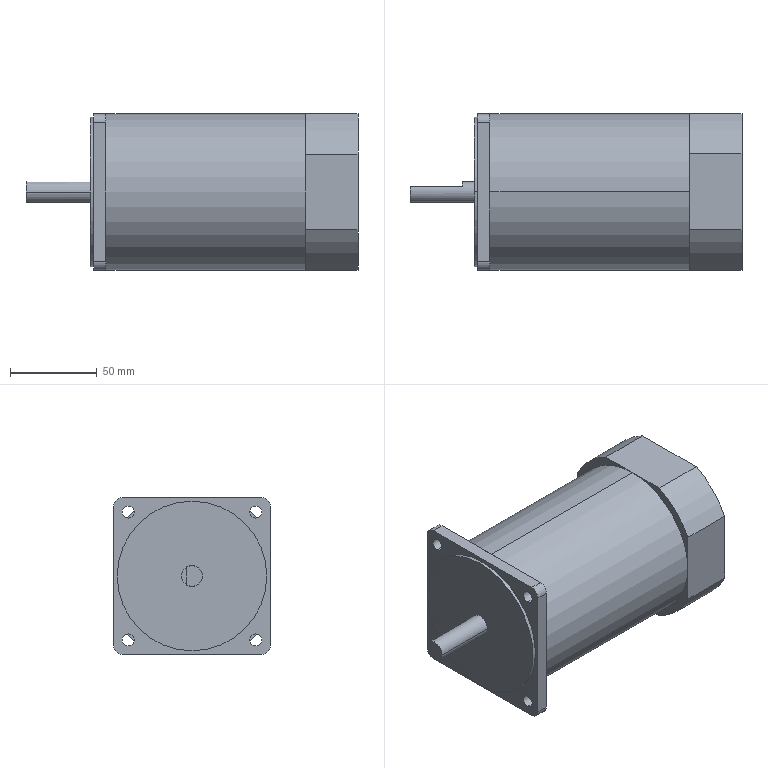Part | STEP file | Motor TWT 5IK60A-C | 1 solid | 44 faces | box 191 x 90 x 90 mm | volume 1020211 mm3 | cylinder 22 | plane 22 | commonest cylinder face diameters 7 x8 10 x4 100 x4 12 x2 86 x2 90 x2